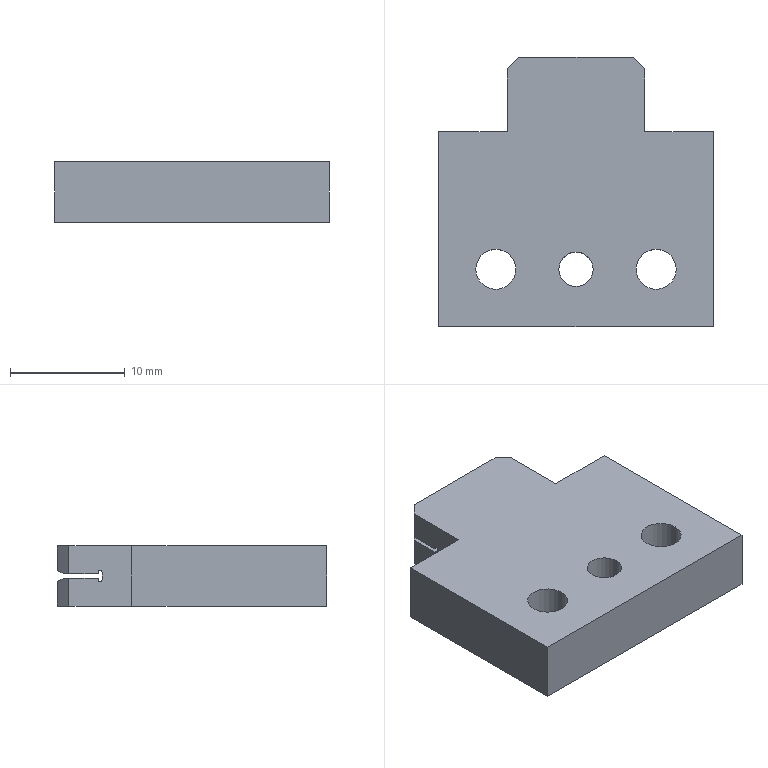Part | NX | 1 solid | 30 faces | box 24 x 23.5 x 5.25 mm | volume 2388 mm3 | plane 22 | cylinder 8 | commonest cylinder face diameters 3.5 x4 0.35 x2 3 x2
STEP:
#1=CARTESIAN_POINT('',(12.,-57.5,8.25));
#2=VERTEX_POINT('',#1);
#3=CARTESIAN_POINT('',(12.,-57.5,3.));
#4=VERTEX_POINT('',#3);
#5=CARTESIAN_POINT('',(12.,-57.5,0.));
#6=DIRECTION('',(0.,0.,-1.));
#7=VECTOR('',#6,1000.);
#8=LINE('',#5,#7);
#9=EDGE_CURVE('',#2,#4,#8,.T.);
#10=ORIENTED_EDGE('',*,*,#9,.F.);
#11=CARTESIAN_POINT('',(-12.,-57.5,8.25));
#12=VERTEX_POINT('',#11);
#13=CARTESIAN_POINT('',(0.,-57.5,8.25));
#14=DIRECTION('',(-1.,0.,0.));
#15=VECTOR('',#14,1000.);
#16=LINE('',#13,#15);
#17=EDGE_CURVE('',#2,#12,#16,.T.);
#18=ORIENTED_EDGE('',*,*,#17,.T.);
#19=CARTESIAN_POINT('',(-12.,-57.5,3.));
#20=VERTEX_POINT('',#19);
#21=CARTESIAN_POINT('',(-12.,-57.5,0.));
#22=DIRECTION('',(0.,0.,1.));
#23=VECTOR('',#22,1000.);
#24=LINE('',#21,#23);
#25=EDGE_CURVE('',#20,#12,#24,.T.);
#26=ORIENTED_EDGE('',*,*,#25,.F.);
#27=CARTESIAN_POINT('',(0.,-57.5,3.));
#28=DIRECTION('',(-1.,0.,0.));
#29=VECTOR('',#28,1000.);
#30=LINE('',#27,#29);
#31=EDGE_CURVE('',#4,#20,#30,.T.);
#32=ORIENTED_EDGE('',*,*,#31,.F.);
#33=EDGE_LOOP('',(#10,#18,#26,#32));
#34=FACE_BOUND('',#33,.T.);
#35=CARTESIAN_POINT('',(-8.,-57.5,0.000000001));
#36=DIRECTION('',(0.,-1.,0.));
#37=DIRECTION('',(0.,0.,-1.));
#38=AXIS2_PLACEMENT_3D('',#35,#36,#37);
#39=PLANE('',#38);
#40=ADVANCED_FACE('',(#34),#39,.T.);
#41=CARTESIAN_POINT('',(6.,-35.,5.45));
#42=VERTEX_POINT('',#41);
#43=CARTESIAN_POINT('',(6.,-35.,3.));
#44=VERTEX_POINT('',#43);
#45=CARTESIAN_POINT('',(6.,-35.,0.));
#46=DIRECTION('',(0.,0.,-1.));
#47=VECTOR('',#46,1000.);
#48=LINE('',#45,#47);
#49=EDGE_CURVE('',#42,#44,#48,.T.);
#50=ORIENTED_EDGE('',*,*,#49,.T.);
#51=CARTESIAN_POINT('',(5.,-34.,3.));
#52=VERTEX_POINT('',#51);
#53=CARTESIAN_POINT('',(-29.,0.,3.));
#54=DIRECTION('',(0.7071,-0.7071,0.));
#55=VECTOR('',#54,1000.);
#56=LINE('',#53,#55);
#57=EDGE_CURVE('',#52,#44,#56,.T.);
#58=ORIENTED_EDGE('',*,*,#57,.F.);
#59=CARTESIAN_POINT('',(5.,-34.,5.15));
#60=VERTEX_POINT('',#59);
#61=CARTESIAN_POINT('',(5.,-34.,0.));
#62=DIRECTION('',(0.,0.,-1.));
#63=VECTOR('',#62,1000.);
#64=LINE('',#61,#63);
#65=EDGE_CURVE('',#60,#52,#64,.T.);
#66=ORIENTED_EDGE('',*,*,#65,.F.);
#67=CARTESIAN_POINT('',(5.6,-34.6,5.45));
#68=VERTEX_POINT('',#67);
#69=CARTESIAN_POINT('',(-29.,0.,-11.85));
#70=DIRECTION('',(0.6667,-0.6667,0.3333));
#71=VECTOR('',#70,1000.);
#72=LINE('',#69,#71);
#73=EDGE_CURVE('',#60,#68,#72,.T.);
#74=ORIENTED_EDGE('',*,*,#73,.T.);
#75=CARTESIAN_POINT('',(-29.,0.,5.45));
#76=DIRECTION('',(-0.7071,0.7071,0.));
#77=VECTOR('',#76,1000.);
#78=LINE('',#75,#77);
#79=EDGE_CURVE('',#42,#68,#78,.T.);
#80=ORIENTED_EDGE('',*,*,#79,.F.);
#81=EDGE_LOOP('',(#50,#58,#66,#74,#80));
#82=FACE_BOUND('',#81,.T.);
#83=CARTESIAN_POINT('',(5.5,-34.5,4.075));
#84=DIRECTION('',(0.7071,0.7071,0.));
#85=DIRECTION('',(0.,0.,-1.));
#86=AXIS2_PLACEMENT_3D('',#83,#84,#85);
#87=PLANE('',#86);
#88=ADVANCED_FACE('',(#82),#87,.T.);
#89=ORIENTED_EDGE('',*,*,#25,.T.);
#90=CARTESIAN_POINT('',(-12.,-40.5,8.25));
#91=VERTEX_POINT('',#90);
#92=CARTESIAN_POINT('',(-12.,0.,8.25));
#93=DIRECTION('',(0.,1.,0.));
#94=VECTOR('',#93,1000.);
#95=LINE('',#92,#94);
#96=EDGE_CURVE('',#12,#91,#95,.T.);
#97=ORIENTED_EDGE('',*,*,#96,.T.);
#98=CARTESIAN_POINT('',(-12.,-40.5,3.));
#99=VERTEX_POINT('',#98);
#100=CARTESIAN_POINT('',(-12.,-40.5,0.));
#101=DIRECTION('',(0.,0.,1.));
#102=VECTOR('',#101,1000.);
#103=LINE('',#100,#102);
#104=EDGE_CURVE('',#99,#91,#103,.T.);
#105=ORIENTED_EDGE('',*,*,#104,.F.);
#106=CARTESIAN_POINT('',(-12.,0.,3.));
#107=DIRECTION('',(0.,1.,0.));
#108=VECTOR('',#107,1000.);
#109=LINE('',#106,#108);
#110=EDGE_CURVE('',#20,#99,#109,.T.);
#111=ORIENTED_EDGE('',*,*,#110,.F.);
#112=EDGE_LOOP('',(#89,#97,#105,#111));
#113=FACE_BOUND('',#112,.T.);
#114=CARTESIAN_POINT('',(-12.,9.5,0.000000001));
#115=DIRECTION('',(-1.,0.,0.));
#116=DIRECTION('',(0.,0.,1.));
#117=AXIS2_PLACEMENT_3D('',#114,#115,#116);
#118=PLANE('',#117);
#119=ADVANCED_FACE('',(#113),#118,.T.);
#120=CARTESIAN_POINT('',(12.,-40.5,8.25));
#121=VERTEX_POINT('',#120);
#122=CARTESIAN_POINT('',(12.,0.,8.25));
#123=DIRECTION('',(0.,-1.,0.));
#124=VECTOR('',#123,1000.);
#125=LINE('',#122,#124);
#126=EDGE_CURVE('',#121,#2,#125,.T.);
#127=ORIENTED_EDGE('',*,*,#126,.F.);
#128=CARTESIAN_POINT('',(6.,-40.5,8.25));
#129=VERTEX_POINT('',#128);
#130=CARTESIAN_POINT('',(0.,-40.5,8.25));
#131=DIRECTION('',(-1.,0.,0.));
#132=VECTOR('',#131,1000.);
#133=LINE('',#130,#132);
#134=EDGE_CURVE('',#121,#129,#133,.T.);
#135=ORIENTED_EDGE('',*,*,#134,.T.);
#136=CARTESIAN_POINT('',(6.,-35.,8.25));
#137=VERTEX_POINT('',#136);
#138=CARTESIAN_POINT('',(6.,0.,8.25));
#139=DIRECTION('',(0.,1.,0.));
#140=VECTOR('',#139,1000.);
#141=LINE('',#138,#140);
#142=EDGE_CURVE('',#129,#137,#141,.T.);
#143=ORIENTED_EDGE('',*,*,#142,.T.);
#144=CARTESIAN_POINT('',(5.,-34.,8.25));
#145=VERTEX_POINT('',#144);
#146=CARTESIAN_POINT('',(-29.,0.,8.25));
#147=DIRECTION('',(0.7071,-0.7071,0.));
#148=VECTOR('',#147,1000.);
#149=LINE('',#146,#148);
#150=EDGE_CURVE('',#145,#137,#149,.T.);
#151=ORIENTED_EDGE('',*,*,#150,.F.);
#152=CARTESIAN_POINT('',(-5.,-34.,8.25));
#153=VERTEX_POINT('',#152);
#154=CARTESIAN_POINT('',(0.,-34.,8.25));
#155=DIRECTION('',(-1.,0.,0.));
#156=VECTOR('',#155,1000.);
#157=LINE('',#154,#156);
#158=EDGE_CURVE('',#145,#153,#157,.T.);
#159=ORIENTED_EDGE('',*,*,#158,.T.);
#160=CARTESIAN_POINT('',(-6.,-35.,8.25));
#161=VERTEX_POINT('',#160);
#162=CARTESIAN_POINT('',(29.,0.,8.25));
#163=DIRECTION('',(0.7071,0.7071,0.));
#164=VECTOR('',#163,1000.);
#165=LINE('',#162,#164);
#166=EDGE_CURVE('',#161,#153,#165,.T.);
#167=ORIENTED_EDGE('',*,*,#166,.F.);
#168=CARTESIAN_POINT('',(-6.,-40.5,8.25));
#169=VERTEX_POINT('',#168);
#170=CARTESIAN_POINT('',(-6.,0.,8.25));
#171=DIRECTION('',(0.,-1.,0.));
#172=VECTOR('',#171,1000.);
#173=LINE('',#170,#172);
#174=EDGE_CURVE('',#161,#169,#173,.T.);
#175=ORIENTED_EDGE('',*,*,#174,.T.);
#176=CARTESIAN_POINT('',(0.,-40.5,8.25));
#177=DIRECTION('',(-1.,0.,0.));
#178=VECTOR('',#177,1000.);
#179=LINE('',#176,#178);
#180=EDGE_CURVE('',#169,#91,#179,.T.);
#181=ORIENTED_EDGE('',*,*,#180,.T.);
#182=ORIENTED_EDGE('',*,*,#96,.F.);
#183=ORIENTED_EDGE('',*,*,#17,.F.);
#184=EDGE_LOOP('',(#127,#135,#143,#151,#159,#167,#175,#181,#182,#183));
#185=FACE_BOUND('',#184,.T.);
#186=CARTESIAN_POINT('',(1.5,-52.5,8.25));
#187=VERTEX_POINT('',#186);
#188=CARTESIAN_POINT('',(-1.5,-52.5,8.25));
#189=VERTEX_POINT('',#188);
#190=CARTESIAN_POINT('',(0.,-52.5,8.25));
#191=DIRECTION('',(0.,0.,1.));
#192=DIRECTION('',(1.,0.,0.));
#193=AXIS2_PLACEMENT_3D('',#190,#191,#192);
#194=CIRCLE('',#193,1.5);
#195=EDGE_CURVE('',#187,#189,#194,.T.);
#196=ORIENTED_EDGE('',*,*,#195,.F.);
#197=CARTESIAN_POINT('',(0.,-52.5,8.25));
#198=DIRECTION('',(0.,0.,1.));
#199=DIRECTION('',(1.,0.,0.));
#200=AXIS2_PLACEMENT_3D('',#197,#198,#199);
#201=CIRCLE('',#200,1.5);
#202=EDGE_CURVE('',#189,#187,#201,.T.);
#203=ORIENTED_EDGE('',*,*,#202,.F.);
#204=EDGE_LOOP('',(#196,#203));
#205=FACE_BOUND('',#204,.T.);
#206=CARTESIAN_POINT('',(5.25,-52.5,8.25));
#207=VERTEX_POINT('',#206);
#208=CARTESIAN_POINT('',(8.75,-52.5,8.25));
#209=VERTEX_POINT('',#208);
#210=CARTESIAN_POINT('',(7.,-52.5,8.25));
#211=DIRECTION('',(0.,0.,1.));
#212=DIRECTION('',(1.,0.,0.));
#213=AXIS2_PLACEMENT_3D('',#210,#211,#212);
#214=CIRCLE('',#213,1.75);
#215=EDGE_CURVE('',#207,#209,#214,.T.);
#216=ORIENTED_EDGE('',*,*,#215,.F.);
#217=CARTESIAN_POINT('',(7.,-52.5,8.25));
#218=DIRECTION('',(0.,0.,1.));
#219=DIRECTION('',(1.,0.,0.));
#220=AXIS2_PLACEMENT_3D('',#217,#218,#219);
#221=CIRCLE('',#220,1.75);
#222=EDGE_CURVE('',#209,#207,#221,.T.);
#223=ORIENTED_EDGE('',*,*,#222,.F.);
#224=EDGE_LOOP('',(#216,#223));
#225=FACE_BOUND('',#224,.T.);
#226=CARTESIAN_POINT('',(-5.25,-52.5,8.25));
#227=VERTEX_POINT('',#226);
#228=CARTESIAN_POINT('',(-8.75,-52.5,8.25));
#229=VERTEX_POINT('',#228);
#230=CARTESIAN_POINT('',(-7.,-52.5,8.25));
#231=DIRECTION('',(0.,0.,1.));
#232=DIRECTION('',(1.,0.,0.));
#233=AXIS2_PLACEMENT_3D('',#230,#231,#232);
#234=CIRCLE('',#233,1.75);
#235=EDGE_CURVE('',#227,#229,#234,.T.);
#236=ORIENTED_EDGE('',*,*,#235,.F.);
#237=CARTESIAN_POINT('',(-7.,-52.5,8.25));
#238=DIRECTION('',(0.,0.,1.));
#239=DIRECTION('',(1.,0.,0.));
#240=AXIS2_PLACEMENT_3D('',#237,#238,#239);
#241=CIRCLE('',#240,1.75);
#242=EDGE_CURVE('',#229,#227,#241,.T.);
#243=ORIENTED_EDGE('',*,*,#242,.F.);
#244=EDGE_LOOP('',(#236,#243));
#245=FACE_BOUND('',#244,.T.);
#246=CARTESIAN_POINT('',(0.,-38.,8.25));
#247=DIRECTION('',(0.,0.,1.));
#248=DIRECTION('',(1.,0.,0.));
#249=AXIS2_PLACEMENT_3D('',#246,#247,#248);
#250=PLANE('',#249);
#251=ADVANCED_FACE('',(#185,#205,#225,#245),#250,.T.);
#252=CARTESIAN_POINT('',(6.,-35.,5.8));
#253=VERTEX_POINT('',#252);
#254=CARTESIAN_POINT('',(6.,-35.,0.));
#255=DIRECTION('',(0.,0.,-1.));
#256=VECTOR('',#255,1000.);
#257=LINE('',#254,#256);
#258=EDGE_CURVE('',#137,#253,#257,.T.);
#259=ORIENTED_EDGE('',*,*,#258,.T.);
#260=CARTESIAN_POINT('',(5.6,-34.6,5.8));
#261=VERTEX_POINT('',#260);
#262=CARTESIAN_POINT('',(-29.,0.,5.8));
#263=DIRECTION('',(0.7071,-0.7071,0.));
#264=VECTOR('',#263,1000.);
#265=LINE('',#262,#264);
#266=EDGE_CURVE('',#261,#253,#265,.T.);
#267=ORIENTED_EDGE('',*,*,#266,.F.);
#268=CARTESIAN_POINT('',(5.,-34.,6.1));
#269=VERTEX_POINT('',#268);
#270=CARTESIAN_POINT('',(-29.,0.,23.1));
#271=DIRECTION('',(0.6667,-0.6667,-0.3333));
#272=VECTOR('',#271,1000.);
#273=LINE('',#270,#272);
#274=EDGE_CURVE('',#269,#261,#273,.T.);
#275=ORIENTED_EDGE('',*,*,#274,.F.);
#276=CARTESIAN_POINT('',(5.,-34.,0.));
#277=DIRECTION('',(0.,0.,-1.));
#278=VECTOR('',#277,1000.);
#279=LINE('',#276,#278);
#280=EDGE_CURVE('',#145,#269,#279,.T.);
#281=ORIENTED_EDGE('',*,*,#280,.F.);
#282=ORIENTED_EDGE('',*,*,#150,.T.);
#283=EDGE_LOOP('',(#259,#267,#275,#281,#282));
#284=FACE_BOUND('',#283,.T.);
#285=CARTESIAN_POINT('',(5.5,-34.5,7.175));
#286=DIRECTION('',(0.7071,0.7071,0.));
#287=DIRECTION('',(0.,0.,-1.));
#288=AXIS2_PLACEMENT_3D('',#285,#286,#287);
#289=PLANE('',#288);
#290=ADVANCED_FACE('',(#284),#289,.T.);
#291=CARTESIAN_POINT('',(-6.,-35.,5.8));
#292=VERTEX_POINT('',#291);
#293=CARTESIAN_POINT('',(-6.,-35.,0.));
#294=DIRECTION('',(0.,0.,1.));
#295=VECTOR('',#294,1000.);
#296=LINE('',#293,#295);
#297=EDGE_CURVE('',#292,#161,#296,.T.);
#298=ORIENTED_EDGE('',*,*,#297,.T.);
#299=ORIENTED_EDGE('',*,*,#166,.T.);
#300=CARTESIAN_POINT('',(-5.,-34.,6.1));
#301=VERTEX_POINT('',#300);
#302=CARTESIAN_POINT('',(-5.,-34.,0.));
#303=DIRECTION('',(0.,0.,1.));
#304=VECTOR('',#303,1000.);
#305=LINE('',#302,#304);
#306=EDGE_CURVE('',#301,#153,#305,.T.);
#307=ORIENTED_EDGE('',*,*,#306,.F.);
#308=CARTESIAN_POINT('',(-5.6,-34.6,5.8));
#309=VERTEX_POINT('',#308);
#310=CARTESIAN_POINT('',(29.,0.,23.1));
#311=DIRECTION('',(0.6667,0.6667,0.3333));
#312=VECTOR('',#311,1000.);
#313=LINE('',#310,#312);
#314=EDGE_CURVE('',#309,#301,#313,.T.);
#315=ORIENTED_EDGE('',*,*,#314,.F.);
#316=CARTESIAN_POINT('',(29.,0.,5.8));
#317=DIRECTION('',(0.7071,0.7071,0.));
#318=VECTOR('',#317,1000.);
#319=LINE('',#316,#318);
#320=EDGE_CURVE('',#292,#309,#319,.T.);
#321=ORIENTED_EDGE('',*,*,#320,.F.);
#322=EDGE_LOOP('',(#298,#299,#307,#315,#321));
#323=FACE_BOUND('',#322,.T.);
#324=CARTESIAN_POINT('',(-5.5,-34.5,7.175));
#325=DIRECTION('',(-0.7071,0.7071,0.));
#326=DIRECTION('',(0.,0.,1.));
#327=AXIS2_PLACEMENT_3D('',#324,#325,#326);
#328=PLANE('',#327);
#329=ADVANCED_FACE('',(#323),#328,.T.);
#330=ORIENTED_EDGE('',*,*,#31,.T.);
#331=ORIENTED_EDGE('',*,*,#110,.T.);
#332=CARTESIAN_POINT('',(-6.,-40.5,3.));
#333=VERTEX_POINT('',#332);
#334=CARTESIAN_POINT('',(0.,-40.5,3.));
#335=DIRECTION('',(-1.,0.,0.));
#336=VECTOR('',#335,1000.);
#337=LINE('',#334,#336);
#338=EDGE_CURVE('',#333,#99,#337,.T.);
#339=ORIENTED_EDGE('',*,*,#338,.F.);
#340=CARTESIAN_POINT('',(-6.,-35.,3.));
#341=VERTEX_POINT('',#340);
#342=CARTESIAN_POINT('',(-6.,0.,3.));
#343=DIRECTION('',(0.,-1.,0.));
#344=VECTOR('',#343,1000.);
#345=LINE('',#342,#344);
#346=EDGE_CURVE('',#341,#333,#345,.T.);
#347=ORIENTED_EDGE('',*,*,#346,.F.);
#348=CARTESIAN_POINT('',(-5.,-34.,3.));
#349=VERTEX_POINT('',#348);
#350=CARTESIAN_POINT('',(29.,0.,3.));
#351=DIRECTION('',(0.7071,0.7071,0.));
#352=VECTOR('',#351,1000.);
#353=LINE('',#350,#352);
#354=EDGE_CURVE('',#341,#349,#353,.T.);
#355=ORIENTED_EDGE('',*,*,#354,.T.);
#356=CARTESIAN_POINT('',(0.,-34.,3.));
#357=DIRECTION('',(-1.,0.,0.));
#358=VECTOR('',#357,1000.);
#359=LINE('',#356,#358);
#360=EDGE_CURVE('',#52,#349,#359,.T.);
#361=ORIENTED_EDGE('',*,*,#360,.F.);
#362=ORIENTED_EDGE('',*,*,#57,.T.);
#363=CARTESIAN_POINT('',(6.,-40.5,3.));
#364=VERTEX_POINT('',#363);
#365=CARTESIAN_POINT('',(6.,0.,3.));
#366=DIRECTION('',(0.,1.,0.));
#367=VECTOR('',#366,1000.);
#368=LINE('',#365,#367);
#369=EDGE_CURVE('',#364,#44,#368,.T.);
#370=ORIENTED_EDGE('',*,*,#369,.F.);
#371=CARTESIAN_POINT('',(12.,-40.5,3.));
#372=VERTEX_POINT('',#371);
#373=CARTESIAN_POINT('',(0.,-40.5,3.));
#374=DIRECTION('',(-1.,0.,0.));
#375=VECTOR('',#374,1000.);
#376=LINE('',#373,#375);
#377=EDGE_CURVE('',#372,#364,#376,.T.);
#378=ORIENTED_EDGE('',*,*,#377,.F.);
#379=CARTESIAN_POINT('',(12.,0.,3.));
#380=DIRECTION('',(0.,-1.,0.));
#381=VECTOR('',#380,1000.);
#382=LINE('',#379,#381);
#383=EDGE_CURVE('',#372,#4,#382,.T.);
#384=ORIENTED_EDGE('',*,*,#383,.T.);
#385=EDGE_LOOP('',(#330,#331,#339,#347,#355,#361,#362,#370,#378,#384));
#386=FACE_BOUND('',#385,.T.);
#387=CARTESIAN_POINT('',(-1.5,-52.5,3.));
#388=VERTEX_POINT('',#387);
#389=CARTESIAN_POINT('',(1.5,-52.5,3.));
#390=VERTEX_POINT('',#389);
#391=CARTESIAN_POINT('',(0.,-52.5,3.));
#392=DIRECTION('',(0.,0.,1.));
#393=DIRECTION('',(1.,0.,0.));
#394=AXIS2_PLACEMENT_3D('',#391,#392,#393);
#395=CIRCLE('',#394,1.5);
#396=EDGE_CURVE('',#388,#390,#395,.T.);
#397=ORIENTED_EDGE('',*,*,#396,.T.);
#398=CARTESIAN_POINT('',(0.,-52.5,3.));
#399=DIRECTION('',(0.,0.,1.));
#400=DIRECTION('',(1.,0.,0.));
#401=AXIS2_PLACEMENT_3D('',#398,#399,#400);
#402=CIRCLE('',#401,1.5);
#403=EDGE_CURVE('',#390,#388,#402,.T.);
#404=ORIENTED_EDGE('',*,*,#403,.T.);
#405=EDGE_LOOP('',(#397,#404));
#406=FACE_BOUND('',#405,.T.);
#407=CARTESIAN_POINT('',(-8.75,-52.5,3.));
#408=VERTEX_POINT('',#407);
#409=CARTESIAN_POINT('',(-5.25,-52.5,3.));
#410=VERTEX_POINT('',#409);
#411=CARTESIAN_POINT('',(-7.,-52.5,3.));
#412=DIRECTION('',(0.,0.,1.));
#413=DIRECTION('',(1.,0.,0.));
#414=AXIS2_PLACEMENT_3D('',#411,#412,#413);
#415=CIRCLE('',#414,1.75);
#416=EDGE_CURVE('',#408,#410,#415,.T.);
#417=ORIENTED_EDGE('',*,*,#416,.T.);
#418=CARTESIAN_POINT('',(-7.,-52.5,3.));
#419=DIRECTION('',(0.,0.,1.));
#420=DIRECTION('',(1.,0.,0.));
#421=AXIS2_PLACEMENT_3D('',#418,#419,#420);
#422=CIRCLE('',#421,1.75);
#423=EDGE_CURVE('',#410,#408,#422,.T.);
#424=ORIENTED_EDGE('',*,*,#423,.T.);
#425=EDGE_LOOP('',(#417,#424));
#426=FACE_BOUND('',#425,.T.);
#427=CARTESIAN_POINT('',(5.25,-52.5,3.));
#428=VERTEX_POINT('',#427);
#429=CARTESIAN_POINT('',(8.75,-52.5,3.));
#430=VERTEX_POINT('',#429);
#431=CARTESIAN_POINT('',(7.,-52.5,3.));
#432=DIRECTION('',(0.,0.,1.));
#433=DIRECTION('',(1.,0.,0.));
#434=AXIS2_PLACEMENT_3D('',#431,#432,#433);
#435=CIRCLE('',#434,1.75);
#436=EDGE_CURVE('',#428,#430,#435,.T.);
#437=ORIENTED_EDGE('',*,*,#436,.T.);
#438=CARTESIAN_POINT('',(7.,-52.5,3.));
#439=DIRECTION('',(0.,0.,1.));
#440=DIRECTION('',(1.,0.,0.));
#441=AXIS2_PLACEMENT_3D('',#438,#439,#440);
#442=CIRCLE('',#441,1.75);
#443=EDGE_CURVE('',#430,#428,#442,.T.);
#444=ORIENTED_EDGE('',*,*,#443,.T.);
#445=EDGE_LOOP('',(#437,#444));
#446=FACE_BOUND('',#445,.T.);
#447=CARTESIAN_POINT('',(-8.,-38.,3.));
#448=DIRECTION('',(0.,0.,1.));
#449=DIRECTION('',(1.,0.,0.));
#450=AXIS2_PLACEMENT_3D('',#447,#448,#449);
#451=PLANE('',#450);
#452=ADVANCED_FACE('',(#386,#406,#426,#446),#451,.F.);
#453=ORIENTED_EDGE('',*,*,#9,.T.);
#454=ORIENTED_EDGE('',*,*,#383,.F.);
#455=CARTESIAN_POINT('',(12.,-40.5,0.));
#456=DIRECTION('',(0.,0.,-1.));
#457=VECTOR('',#456,1000.);
#458=LINE('',#455,#457);
#459=EDGE_CURVE('',#121,#372,#458,.T.);
#460=ORIENTED_EDGE('',*,*,#459,.F.);
#461=ORIENTED_EDGE('',*,*,#126,.T.);
#462=EDGE_LOOP('',(#453,#454,#460,#461));
#463=FACE_BOUND('',#462,.T.);
#464=CARTESIAN_POINT('',(12.,-38.,0.000000001));
#465=DIRECTION('',(1.,0.,0.));
#466=DIRECTION('',(0.,1.,0.));
#467=AXIS2_PLACEMENT_3D('',#464,#465,#466);
#468=PLANE('',#467);
#469=ADVANCED_FACE('',(#463),#468,.T.);
#470=CARTESIAN_POINT('',(-6.,-35.,5.45));
#471=VERTEX_POINT('',#470);
#472=CARTESIAN_POINT('',(-6.,-35.,0.));
#473=DIRECTION('',(0.,0.,1.));
#474=VECTOR('',#473,1000.);
#475=LINE('',#472,#474);
#476=EDGE_CURVE('',#341,#471,#475,.T.);
#477=ORIENTED_EDGE('',*,*,#476,.T.);
#478=CARTESIAN_POINT('',(-5.6,-34.6,5.45));
#479=VERTEX_POINT('',#478);
#480=CARTESIAN_POINT('',(29.,0.,5.45));
#481=DIRECTION('',(-0.7071,-0.7071,0.));
#482=VECTOR('',#481,1000.);
#483=LINE('',#480,#482);
#484=EDGE_CURVE('',#479,#471,#483,.T.);
#485=ORIENTED_EDGE('',*,*,#484,.F.);
#486=CARTESIAN_POINT('',(-5.,-34.,5.15));
#487=VERTEX_POINT('',#486);
#488=CARTESIAN_POINT('',(29.,0.,-11.85));
#489=DIRECTION('',(0.6667,0.6667,-0.3333));
#490=VECTOR('',#489,1000.);
#491=LINE('',#488,#490);
#492=EDGE_CURVE('',#479,#487,#491,.T.);
#493=ORIENTED_EDGE('',*,*,#492,.T.);
#494=CARTESIAN_POINT('',(-5.,-34.,0.));
#495=DIRECTION('',(0.,0.,1.));
#496=VECTOR('',#495,1000.);
#497=LINE('',#494,#496);
#498=EDGE_CURVE('',#349,#487,#497,.T.);
#499=ORIENTED_EDGE('',*,*,#498,.F.);
#500=ORIENTED_EDGE('',*,*,#354,.F.);
#501=EDGE_LOOP('',(#477,#485,#493,#499,#500));
#502=FACE_BOUND('',#501,.T.);
#503=CARTESIAN_POINT('',(-5.5,-34.5,4.075));
#504=DIRECTION('',(-0.7071,0.7071,0.));
#505=DIRECTION('',(0.,0.,1.));
#506=AXIS2_PLACEMENT_3D('',#503,#504,#505);
#507=PLANE('',#506);
#508=ADVANCED_FACE('',(#502),#507,.T.);
#509=ORIENTED_EDGE('',*,*,#306,.T.);
#510=ORIENTED_EDGE('',*,*,#158,.F.);
#511=ORIENTED_EDGE('',*,*,#280,.T.);
#512=CARTESIAN_POINT('',(0.,-34.,6.1));
#513=DIRECTION('',(1.,0.,0.));
#514=VECTOR('',#513,1000.);
#515=LINE('',#512,#514);
#516=EDGE_CURVE('',#301,#269,#515,.T.);
#517=ORIENTED_EDGE('',*,*,#516,.F.);
#518=EDGE_LOOP('',(#509,#510,#511,#517));
#519=FACE_BOUND('',#518,.T.);
#520=CARTESIAN_POINT('',(10.8,-34.,30.936));
#521=DIRECTION('',(0.,-1.,0.));
#522=DIRECTION('',(0.,0.,-1.));
#523=AXIS2_PLACEMENT_3D('',#520,#521,#522);
#524=PLANE('',#523);
#525=ADVANCED_FACE('',(#519),#524,.F.);
#526=ORIENTED_EDGE('',*,*,#134,.F.);
#527=ORIENTED_EDGE('',*,*,#459,.T.);
#528=ORIENTED_EDGE('',*,*,#377,.T.);
#529=CARTESIAN_POINT('',(6.,-40.5,0.));
#530=DIRECTION('',(0.,0.,1.));
#531=VECTOR('',#530,1000.);
#532=LINE('',#529,#531);
#533=EDGE_CURVE('',#364,#129,#532,.T.);
#534=ORIENTED_EDGE('',*,*,#533,.T.);
#535=EDGE_LOOP('',(#526,#527,#528,#534));
#536=FACE_BOUND('',#535,.T.);
#537=CARTESIAN_POINT('',(12.,-40.5,2.5));
#538=DIRECTION('',(0.,-1.,0.));
#539=DIRECTION('',(0.,0.,-1.));
#540=AXIS2_PLACEMENT_3D('',#537,#538,#539);
#541=PLANE('',#540);
#542=ADVANCED_FACE('',(#536),#541,.F.);
#543=ORIENTED_EDGE('',*,*,#180,.F.);
#544=CARTESIAN_POINT('',(-6.,-40.5,0.));
#545=DIRECTION('',(0.,0.,-1.));
#546=VECTOR('',#545,1000.);
#547=LINE('',#544,#546);
#548=EDGE_CURVE('',#169,#333,#547,.T.);
#549=ORIENTED_EDGE('',*,*,#548,.T.);
#550=ORIENTED_EDGE('',*,*,#338,.T.);
#551=ORIENTED_EDGE('',*,*,#104,.T.);
#552=EDGE_LOOP('',(#543,#549,#550,#551));
#553=FACE_BOUND('',#552,.T.);
#554=CARTESIAN_POINT('',(-6.,-40.5,2.5));
#555=DIRECTION('',(0.,-1.,0.));
#556=DIRECTION('',(0.,0.,-1.));
#557=AXIS2_PLACEMENT_3D('',#554,#555,#556);
#558=PLANE('',#557);
#559=ADVANCED_FACE('',(#553),#558,.F.);
#560=ORIENTED_EDGE('',*,*,#297,.F.);
#561=CARTESIAN_POINT('',(-6.,-37.55,5.8));
#562=VERTEX_POINT('',#561);
#563=CARTESIAN_POINT('',(-6.,0.,5.8));
#564=DIRECTION('',(0.,-1.,0.));
#565=VECTOR('',#564,1000.);
#566=LINE('',#563,#565);
#567=EDGE_CURVE('',#292,#562,#566,.T.);
#568=ORIENTED_EDGE('',*,*,#567,.T.);
#569=CARTESIAN_POINT('',(-6.,-37.55,5.925));
#570=VERTEX_POINT('',#569);
#571=CARTESIAN_POINT('',(-6.,-37.55,0.));
#572=DIRECTION('',(0.,0.,1.));
#573=VECTOR('',#572,1000.);
#574=LINE('',#571,#573);
#575=EDGE_CURVE('',#562,#570,#574,.T.);
#576=ORIENTED_EDGE('',*,*,#575,.T.);
#577=CARTESIAN_POINT('',(-6.,-37.9,5.925));
#578=VERTEX_POINT('',#577);
#579=CARTESIAN_POINT('',(-6.,-37.725,5.925));
#580=DIRECTION('',(-1.,0.,0.));
#581=DIRECTION('',(0.,0.,1.));
#582=AXIS2_PLACEMENT_3D('',#579,#580,#581);
#583=CIRCLE('',#582,0.175);
#584=EDGE_CURVE('',#578,#570,#583,.T.);
#585=ORIENTED_EDGE('',*,*,#584,.F.);
#586=CARTESIAN_POINT('',(-6.,-37.9,5.325));
#587=VERTEX_POINT('',#586);
#588=CARTESIAN_POINT('',(-6.,-37.9,0.));
#589=DIRECTION('',(0.,0.,-1.));
#590=VECTOR('',#589,1000.);
#591=LINE('',#588,#590);
#592=EDGE_CURVE('',#578,#587,#591,.T.);
#593=ORIENTED_EDGE('',*,*,#592,.T.);
#594=CARTESIAN_POINT('',(-6.,-37.55,5.325));
#595=VERTEX_POINT('',#594);
#596=CARTESIAN_POINT('',(-6.,-37.725,5.325));
#597=DIRECTION('',(-1.,0.,0.));
#598=DIRECTION('',(0.,0.,1.));
#599=AXIS2_PLACEMENT_3D('',#596,#597,#598);
#600=CIRCLE('',#599,0.175);
#601=EDGE_CURVE('',#595,#587,#600,.T.);
#602=ORIENTED_EDGE('',*,*,#601,.F.);
#603=CARTESIAN_POINT('',(-6.,-37.55,5.45));
#604=VERTEX_POINT('',#603);
#605=CARTESIAN_POINT('',(-6.,-37.55,0.));
#606=DIRECTION('',(0.,0.,1.));
#607=VECTOR('',#606,1000.);
#608=LINE('',#605,#607);
#609=EDGE_CURVE('',#595,#604,#608,.T.);
#610=ORIENTED_EDGE('',*,*,#609,.T.);
#611=CARTESIAN_POINT('',(-6.,0.,5.45));
#612=DIRECTION('',(0.,1.,0.));
#613=VECTOR('',#612,1000.);
#614=LINE('',#611,#613);
#615=EDGE_CURVE('',#604,#471,#614,.T.);
#616=ORIENTED_EDGE('',*,*,#615,.T.);
#617=ORIENTED_EDGE('',*,*,#476,.F.);
#618=ORIENTED_EDGE('',*,*,#346,.T.);
#619=ORIENTED_EDGE('',*,*,#548,.F.);
#620=ORIENTED_EDGE('',*,*,#174,.F.);
#621=EDGE_LOOP('',(#560,#568,#576,#585,#593,#602,#610,#616,#617,#618,#619,#620));
#622=FACE_BOUND('',#621,.T.);
#623=CARTESIAN_POINT('',(-6.,-37.5,2.5));
#624=DIRECTION('',(1.,0.,0.));
#625=DIRECTION('',(0.,1.,0.));
#626=AXIS2_PLACEMENT_3D('',#623,#624,#625);
#627=PLANE('',#626);
#628=ADVANCED_FACE('',(#622),#627,.F.);
#629=ORIENTED_EDGE('',*,*,#258,.F.);
#630=ORIENTED_EDGE('',*,*,#142,.F.);
#631=ORIENTED_EDGE('',*,*,#533,.F.);
#632=ORIENTED_EDGE('',*,*,#369,.T.);
#633=ORIENTED_EDGE('',*,*,#49,.F.);
#634=CARTESIAN_POINT('',(6.,-37.55,5.45));
#635=VERTEX_POINT('',#634);
#636=CARTESIAN_POINT('',(6.,0.,5.45));
#637=DIRECTION('',(0.,-1.,0.));
#638=VECTOR('',#637,1000.);
#639=LINE('',#636,#638);
#640=EDGE_CURVE('',#42,#635,#639,.T.);
#641=ORIENTED_EDGE('',*,*,#640,.T.);
#642=CARTESIAN_POINT('',(6.,-37.55,5.325));
#643=VERTEX_POINT('',#642);
#644=CARTESIAN_POINT('',(6.,-37.55,0.));
#645=DIRECTION('',(0.,0.,-1.));
#646=VECTOR('',#645,1000.);
#647=LINE('',#644,#646);
#648=EDGE_CURVE('',#635,#643,#647,.T.);
#649=ORIENTED_EDGE('',*,*,#648,.T.);
#650=CARTESIAN_POINT('',(6.,-37.9,5.325));
#651=VERTEX_POINT('',#650);
#652=CARTESIAN_POINT('',(6.,-37.725,5.325));
#653=DIRECTION('',(-1.,0.,0.));
#654=DIRECTION('',(0.,1.,0.));
#655=AXIS2_PLACEMENT_3D('',#652,#653,#654);
#656=CIRCLE('',#655,0.175);
#657=EDGE_CURVE('',#643,#651,#656,.T.);
#658=ORIENTED_EDGE('',*,*,#657,.T.);
#659=CARTESIAN_POINT('',(6.,-37.9,5.925));
#660=VERTEX_POINT('',#659);
#661=CARTESIAN_POINT('',(6.,-37.9,0.));
#662=DIRECTION('',(0.,0.,1.));
#663=VECTOR('',#662,1000.);
#664=LINE('',#661,#663);
#665=EDGE_CURVE('',#651,#660,#664,.T.);
#666=ORIENTED_EDGE('',*,*,#665,.T.);
#667=CARTESIAN_POINT('',(6.,-37.55,5.925));
#668=VERTEX_POINT('',#667);
#669=CARTESIAN_POINT('',(6.,-37.725,5.925));
#670=DIRECTION('',(1.,0.,0.));
#671=DIRECTION('',(0.,-1.,0.));
#672=AXIS2_PLACEMENT_3D('',#669,#670,#671);
#673=CIRCLE('',#672,0.175);
#674=EDGE_CURVE('',#668,#660,#673,.T.);
#675=ORIENTED_EDGE('',*,*,#674,.F.);
#676=CARTESIAN_POINT('',(6.,-37.55,5.8));
#677=VERTEX_POINT('',#676);
#678=CARTESIAN_POINT('',(6.,-37.55,0.));
#679=DIRECTION('',(0.,0.,-1.));
#680=VECTOR('',#679,1000.);
#681=LINE('',#678,#680);
#682=EDGE_CURVE('',#668,#677,#681,.T.);
#683=ORIENTED_EDGE('',*,*,#682,.T.);
#684=CARTESIAN_POINT('',(6.,0.,5.8));
#685=DIRECTION('',(0.,1.,0.));
#686=VECTOR('',#685,1000.);
#687=LINE('',#684,#686);
#688=EDGE_CURVE('',#677,#253,#687,.T.);
#689=ORIENTED_EDGE('',*,*,#688,.T.);
#690=EDGE_LOOP('',(#629,#630,#631,#632,#633,#641,#649,#658,#666,#675,#683,#689));
#691=FACE_BOUND('',#690,.T.);
#692=CARTESIAN_POINT('',(6.,-40.5,2.5));
#693=DIRECTION('',(-1.,0.,0.));
#694=DIRECTION('',(0.,0.,1.));
#695=AXIS2_PLACEMENT_3D('',#692,#693,#694);
#696=PLANE('',#695);
#697=ADVANCED_FACE('',(#691),#696,.F.);
#698=ORIENTED_EDGE('',*,*,#65,.T.);
#699=ORIENTED_EDGE('',*,*,#360,.T.);
#700=ORIENTED_EDGE('',*,*,#498,.T.);
#701=CARTESIAN_POINT('',(0.,-34.,5.15));
#702=DIRECTION('',(1.,0.,0.));
#703=VECTOR('',#702,1000.);
#704=LINE('',#701,#703);
#705=EDGE_CURVE('',#487,#60,#704,.T.);
#706=ORIENTED_EDGE('',*,*,#705,.T.);
#707=EDGE_LOOP('',(#698,#699,#700,#706));
#708=FACE_BOUND('',#707,.T.);
#709=CARTESIAN_POINT('',(10.8,-34.,30.936));
#710=DIRECTION('',(0.,-1.,0.));
#711=DIRECTION('',(0.,0.,-1.));
#712=AXIS2_PLACEMENT_3D('',#709,#710,#711);
#713=PLANE('',#712);
#714=ADVANCED_FACE('',(#708),#713,.F.);
#715=CARTESIAN_POINT('',(0.,-34.6,5.8));
#716=DIRECTION('',(-1.,0.,0.));
#717=VECTOR('',#716,1000.);
#718=LINE('',#715,#717);
#719=EDGE_CURVE('',#261,#309,#718,.T.);
#720=ORIENTED_EDGE('',*,*,#719,.F.);
#721=ORIENTED_EDGE('',*,*,#266,.T.);
#722=ORIENTED_EDGE('',*,*,#688,.F.);
#723=CARTESIAN_POINT('',(0.,-37.55,5.8));
#724=DIRECTION('',(-1.,0.,0.));
#725=VECTOR('',#724,1000.);
#726=LINE('',#723,#725);
#727=EDGE_CURVE('',#677,#562,#726,.T.);
#728=ORIENTED_EDGE('',*,*,#727,.T.);
#729=ORIENTED_EDGE('',*,*,#567,.F.);
#730=ORIENTED_EDGE('',*,*,#320,.T.);
#731=EDGE_LOOP('',(#720,#721,#722,#728,#729,#730));
#732=FACE_BOUND('',#731,.T.);
#733=CARTESIAN_POINT('',(-14.4,-37.5,5.8));
#734=DIRECTION('',(0.,0.,1.));
#735=DIRECTION('',(1.,0.,0.));
#736=AXIS2_PLACEMENT_3D('',#733,#734,#735);
#737=PLANE('',#736);
#738=ADVANCED_FACE('',(#732),#737,.F.);
#739=CARTESIAN_POINT('',(0.,-37.55,5.925));
#740=DIRECTION('',(1.,0.,0.));
#741=VECTOR('',#740,1000.);
#742=LINE('',#739,#741);
#743=EDGE_CURVE('',#570,#668,#742,.T.);
#744=ORIENTED_EDGE('',*,*,#743,.T.);
#745=ORIENTED_EDGE('',*,*,#674,.T.);
#746=CARTESIAN_POINT('',(0.,-37.9,5.925));
#747=DIRECTION('',(1.,0.,0.));
#748=VECTOR('',#747,1000.);
#749=LINE('',#746,#748);
#750=EDGE_CURVE('',#578,#660,#749,.T.);
#751=ORIENTED_EDGE('',*,*,#750,.F.);
#752=ORIENTED_EDGE('',*,*,#584,.T.);
#753=EDGE_LOOP('',(#744,#745,#751,#752));
#754=FACE_BOUND('',#753,.T.);
#755=CARTESIAN_POINT('',(-7.2,-37.725,5.925));
#756=DIRECTION('',(1.,0.,0.));
#757=DIRECTION('',(0.,-1.,0.));
#758=AXIS2_PLACEMENT_3D('',#755,#756,#757);
#759=CYLINDRICAL_SURFACE('',#758,0.175);
#760=ADVANCED_FACE('',(#754),#759,.F.);
#761=CARTESIAN_POINT('',(0.,-34.6,5.45));
#762=DIRECTION('',(1.,0.,0.));
#763=VECTOR('',#762,1000.);
#764=LINE('',#761,#763);
#765=EDGE_CURVE('',#479,#68,#764,.T.);
#766=ORIENTED_EDGE('',*,*,#765,.F.);
#767=ORIENTED_EDGE('',*,*,#484,.T.);
#768=ORIENTED_EDGE('',*,*,#615,.F.);
#769=CARTESIAN_POINT('',(0.,-37.55,5.45));
#770=DIRECTION('',(1.,0.,0.));
#771=VECTOR('',#770,1000.);
#772=LINE('',#769,#771);
#773=EDGE_CURVE('',#604,#635,#772,.T.);
#774=ORIENTED_EDGE('',*,*,#773,.T.);
#775=ORIENTED_EDGE('',*,*,#640,.F.);
#776=ORIENTED_EDGE('',*,*,#79,.T.);
#777=EDGE_LOOP('',(#766,#767,#768,#774,#775,#776));
#778=FACE_BOUND('',#777,.T.);
#779=CARTESIAN_POINT('',(-14.4,-34.5,5.45));
#780=DIRECTION('',(0.,0.,-1.));
#781=DIRECTION('',(0.,-1.,0.));
#782=AXIS2_PLACEMENT_3D('',#779,#780,#781);
#783=PLANE('',#782);
#784=ADVANCED_FACE('',(#778),#783,.F.);
#785=ORIENTED_EDGE('',*,*,#719,.T.);
#786=ORIENTED_EDGE('',*,*,#314,.T.);
#787=ORIENTED_EDGE('',*,*,#516,.T.);
#788=ORIENTED_EDGE('',*,*,#274,.T.);
#789=EDGE_LOOP('',(#785,#786,#787,#788));
#790=FACE_BOUND('',#789,.T.);
#791=CARTESIAN_POINT('',(0.,-34.3,5.95));
#792=DIRECTION('',(0.,-0.4472,0.8944));
#793=DIRECTION('',(-1.,0.,0.));
#794=AXIS2_PLACEMENT_3D('',#791,#792,#793);
#795=PLANE('',#794);
#796=ADVANCED_FACE('',(#790),#795,.F.);
#797=ORIENTED_EDGE('',*,*,#765,.T.);
#798=ORIENTED_EDGE('',*,*,#73,.F.);
#799=ORIENTED_EDGE('',*,*,#705,.F.);
#800=ORIENTED_EDGE('',*,*,#492,.F.);
#801=EDGE_LOOP('',(#797,#798,#799,#800));
#802=FACE_BOUND('',#801,.T.);
#803=CARTESIAN_POINT('',(0.,-34.3,5.3));
#804=DIRECTION('',(0.,0.4472,0.8944));
#805=DIRECTION('',(1.,0.,0.));
#806=AXIS2_PLACEMENT_3D('',#803,#804,#805);
#807=PLANE('',#806);
#808=ADVANCED_FACE('',(#802),#807,.T.);
#809=ORIENTED_EDGE('',*,*,#396,.F.);
#810=CARTESIAN_POINT('',(-1.5,-52.5,2.475));
#811=DIRECTION('',(0.,0.,1.));
#812=VECTOR('',#811,1000.);
#813=LINE('',#810,#812);
#814=EDGE_CURVE('',#189,#388,#813,.F.);
#815=ORIENTED_EDGE('',*,*,#814,.F.);
#816=ORIENTED_EDGE('',*,*,#202,.T.);
#817=CARTESIAN_POINT('',(1.5,-52.5,2.475));
#818=DIRECTION('',(0.,0.,1.));
#819=VECTOR('',#818,1000.);
#820=LINE('',#817,#819);
#821=EDGE_CURVE('',#187,#390,#820,.F.);
#822=ORIENTED_EDGE('',*,*,#821,.T.);
#823=EDGE_LOOP('',(#809,#815,#816,#822));
#824=FACE_BOUND('',#823,.T.);
#825=CARTESIAN_POINT('',(0.,-52.5,2.475));
#826=DIRECTION('',(0.,0.,1.));
#827=DIRECTION('',(1.,0.,0.));
#828=AXIS2_PLACEMENT_3D('',#825,#826,#827);
#829=CYLINDRICAL_SURFACE('',#828,1.5);
#830=ADVANCED_FACE('',(#824),#829,.F.);
#831=ORIENTED_EDGE('',*,*,#416,.F.);
#832=CARTESIAN_POINT('',(-8.75,-52.5,2.475));
#833=DIRECTION('',(0.,0.,1.));
#834=VECTOR('',#833,1000.);
#835=LINE('',#832,#834);
#836=EDGE_CURVE('',#229,#408,#835,.F.);
#837=ORIENTED_EDGE('',*,*,#836,.F.);
#838=ORIENTED_EDGE('',*,*,#242,.T.);
#839=CARTESIAN_POINT('',(-5.25,-52.5,2.475));
#840=DIRECTION('',(0.,0.,1.));
#841=VECTOR('',#840,1000.);
#842=LINE('',#839,#841);
#843=EDGE_CURVE('',#227,#410,#842,.F.);
#844=ORIENTED_EDGE('',*,*,#843,.T.);
#845=EDGE_LOOP('',(#831,#837,#838,#844));
#846=FACE_BOUND('',#845,.T.);
#847=CARTESIAN_POINT('',(-7.,-52.5,2.475));
#848=DIRECTION('',(0.,0.,1.));
#849=DIRECTION('',(1.,0.,0.));
#850=AXIS2_PLACEMENT_3D('',#847,#848,#849);
#851=CYLINDRICAL_SURFACE('',#850,1.75);
#852=ADVANCED_FACE('',(#846),#851,.F.);
#853=ORIENTED_EDGE('',*,*,#215,.T.);
#854=CARTESIAN_POINT('',(8.75,-52.5,2.475));
#855=DIRECTION('',(0.,0.,1.));
#856=VECTOR('',#855,1000.);
#857=LINE('',#854,#856);
#858=EDGE_CURVE('',#430,#209,#857,.T.);
#859=ORIENTED_EDGE('',*,*,#858,.F.);
#860=ORIENTED_EDGE('',*,*,#436,.F.);
#861=CARTESIAN_POINT('',(5.25,-52.5,2.475));
#862=DIRECTION('',(0.,0.,1.));
#863=VECTOR('',#862,1000.);
#864=LINE('',#861,#863);
#865=EDGE_CURVE('',#428,#207,#864,.T.);
#866=ORIENTED_EDGE('',*,*,#865,.T.);
#867=EDGE_LOOP('',(#853,#859,#860,#866));
#868=FACE_BOUND('',#867,.T.);
#869=CARTESIAN_POINT('',(7.,-52.5,2.475));
#870=DIRECTION('',(0.,0.,1.));
#871=DIRECTION('',(1.,0.,0.));
#872=AXIS2_PLACEMENT_3D('',#869,#870,#871);
#873=CYLINDRICAL_SURFACE('',#872,1.75);
#874=ADVANCED_FACE('',(#868),#873,.F.);
#875=CARTESIAN_POINT('',(0.,-37.55,5.325));
#876=DIRECTION('',(1.,0.,0.));
#877=VECTOR('',#876,1000.);
#878=LINE('',#875,#877);
#879=EDGE_CURVE('',#595,#643,#878,.T.);
#880=ORIENTED_EDGE('',*,*,#879,.T.);
#881=ORIENTED_EDGE('',*,*,#648,.F.);
#882=ORIENTED_EDGE('',*,*,#773,.F.);
#883=ORIENTED_EDGE('',*,*,#609,.F.);
#884=EDGE_LOOP('',(#880,#881,#882,#883));
#885=FACE_BOUND('',#884,.T.);
#886=CARTESIAN_POINT('',(-14.4,-37.55,6.1));
#887=DIRECTION('',(0.,1.,0.));
#888=DIRECTION('',(1.,0.,0.));
#889=AXIS2_PLACEMENT_3D('',#886,#887,#888);
#890=PLANE('',#889);
#891=ADVANCED_FACE('',(#885),#890,.F.);
#892=ORIENTED_EDGE('',*,*,#743,.F.);
#893=ORIENTED_EDGE('',*,*,#575,.F.);
#894=ORIENTED_EDGE('',*,*,#727,.F.);
#895=ORIENTED_EDGE('',*,*,#682,.F.);
#896=EDGE_LOOP('',(#892,#893,#894,#895));
#897=FACE_BOUND('',#896,.T.);
#898=CARTESIAN_POINT('',(-14.4,-37.55,6.1));
#899=DIRECTION('',(0.,1.,0.));
#900=DIRECTION('',(1.,0.,0.));
#901=AXIS2_PLACEMENT_3D('',#898,#899,#900);
#902=PLANE('',#901);
#903=ADVANCED_FACE('',(#897),#902,.F.);
#904=ORIENTED_EDGE('',*,*,#879,.F.);
#905=ORIENTED_EDGE('',*,*,#601,.T.);
#906=CARTESIAN_POINT('',(0.,-37.9,5.325));
#907=DIRECTION('',(1.,0.,0.));
#908=VECTOR('',#907,1000.);
#909=LINE('',#906,#908);
#910=EDGE_CURVE('',#587,#651,#909,.T.);
#911=ORIENTED_EDGE('',*,*,#910,.T.);
#912=ORIENTED_EDGE('',*,*,#657,.F.);
#913=EDGE_LOOP('',(#904,#905,#911,#912));
#914=FACE_BOUND('',#913,.T.);
#915=CARTESIAN_POINT('',(-7.2,-37.725,5.325));
#916=DIRECTION('',(1.,0.,0.));
#917=DIRECTION('',(0.,-1.,0.));
#918=AXIS2_PLACEMENT_3D('',#915,#916,#917);
#919=CYLINDRICAL_SURFACE('',#918,0.175);
#920=ADVANCED_FACE('',(#914),#919,.F.);
#921=ORIENTED_EDGE('',*,*,#910,.F.);
#922=ORIENTED_EDGE('',*,*,#592,.F.);
#923=ORIENTED_EDGE('',*,*,#750,.T.);
#924=ORIENTED_EDGE('',*,*,#665,.F.);
#925=EDGE_LOOP('',(#921,#922,#923,#924));
#926=FACE_BOUND('',#925,.T.);
#927=CARTESIAN_POINT('',(-14.4,-37.9,5.15));
#928=DIRECTION('',(0.,-1.,0.));
#929=DIRECTION('',(0.,0.,-1.));
#930=AXIS2_PLACEMENT_3D('',#927,#928,#929);
#931=PLANE('',#930);
#932=ADVANCED_FACE('',(#926),#931,.F.);
#933=ORIENTED_EDGE('',*,*,#858,.T.);
#934=ORIENTED_EDGE('',*,*,#222,.T.);
#935=ORIENTED_EDGE('',*,*,#865,.F.);
#936=ORIENTED_EDGE('',*,*,#443,.F.);
#937=EDGE_LOOP('',(#933,#934,#935,#936));
#938=FACE_BOUND('',#937,.T.);
#939=CARTESIAN_POINT('',(7.,-52.5,2.475));
#940=DIRECTION('',(0.,0.,1.));
#941=DIRECTION('',(1.,0.,0.));
#942=AXIS2_PLACEMENT_3D('',#939,#940,#941);
#943=CYLINDRICAL_SURFACE('',#942,1.75);
#944=ADVANCED_FACE('',(#938),#943,.F.);
#945=ORIENTED_EDGE('',*,*,#195,.T.);
#946=ORIENTED_EDGE('',*,*,#814,.T.);
#947=ORIENTED_EDGE('',*,*,#403,.F.);
#948=ORIENTED_EDGE('',*,*,#821,.F.);
#949=EDGE_LOOP('',(#945,#946,#947,#948));
#950=FACE_BOUND('',#949,.T.);
#951=CARTESIAN_POINT('',(0.,-52.5,2.475));
#952=DIRECTION('',(0.,0.,1.));
#953=DIRECTION('',(1.,0.,0.));
#954=AXIS2_PLACEMENT_3D('',#951,#952,#953);
#955=CYLINDRICAL_SURFACE('',#954,1.5);
#956=ADVANCED_FACE('',(#950),#955,.F.);
#957=ORIENTED_EDGE('',*,*,#235,.T.);
#958=ORIENTED_EDGE('',*,*,#836,.T.);
#959=ORIENTED_EDGE('',*,*,#423,.F.);
#960=ORIENTED_EDGE('',*,*,#843,.F.);
#961=EDGE_LOOP('',(#957,#958,#959,#960));
#962=FACE_BOUND('',#961,.T.);
#963=CARTESIAN_POINT('',(-7.,-52.5,2.475));
#964=DIRECTION('',(0.,0.,1.));
#965=DIRECTION('',(1.,0.,0.));
#966=AXIS2_PLACEMENT_3D('',#963,#964,#965);
#967=CYLINDRICAL_SURFACE('',#966,1.75);
#968=ADVANCED_FACE('',(#962),#967,.F.);
#969=CLOSED_SHELL('',(#40,#88,#119,#251,#290,#329,#452,#469,#508,#525,#542,#559,#628,#697,#714,#738,#760,#784,#796,#808,#830,#852,#874,#891,#903,#920,#932,#944,#956,#968));
#970=MANIFOLD_SOLID_BREP('',#969);
#971=(LENGTH_UNIT()NAMED_UNIT(*)SI_UNIT(.MILLI.,.METRE.));
#972=UNCERTAINTY_MEASURE_WITH_UNIT(LENGTH_MEASURE(0.00001),#971,'','');
#973=(NAMED_UNIT(*)PLANE_ANGLE_UNIT()SI_UNIT($,.RADIAN.));
#974=(NAMED_UNIT(*)SI_UNIT($,.STERADIAN.)SOLID_ANGLE_UNIT());
#975=(GEOMETRIC_REPRESENTATION_CONTEXT(3)GLOBAL_UNCERTAINTY_ASSIGNED_CONTEXT((#972))GLOBAL_UNIT_ASSIGNED_CONTEXT((#971,#973,#974))REPRESENTATION_CONTEXT('',''));
#976=ADVANCED_BREP_SHAPE_REPRESENTATION('',(#970),#975);